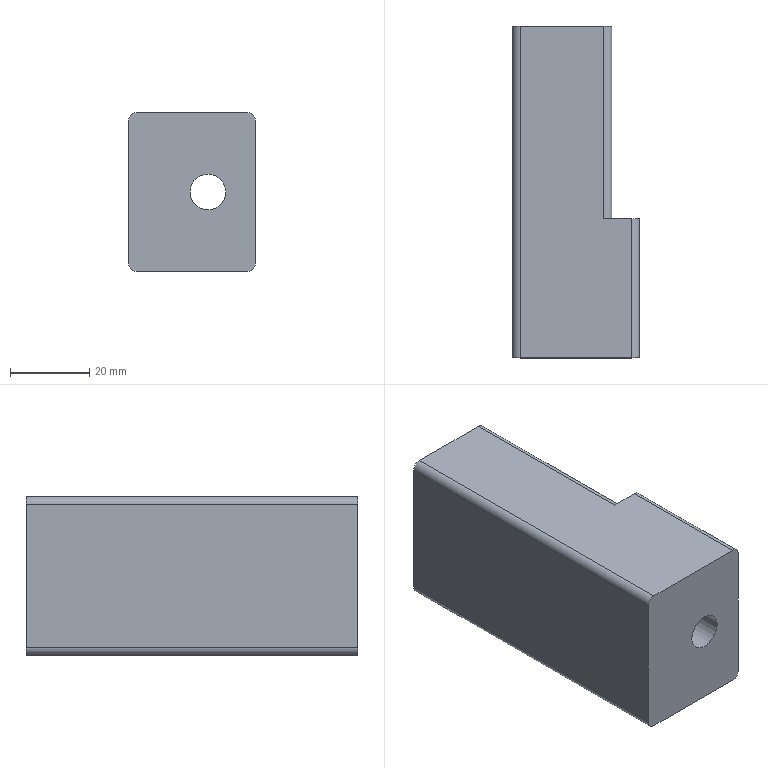CAM job | Mastercam | 3-axis milling, 5-axis milling, drilling | part box 32 x 83.5 x 40 mm | stock box 32 x 90 x 50 mm
Tools:
tool_number,name,type,diameter_mm,corner_radius_mm,flutes,flute_length_mm,overall_length_mm,shoulder_length_mm,holder_diameter_mm,length_offset,diameter_offset,default_rpm,default_feed_mm_min,default_plunge_mm_min,coolant
1,2 Flat End Mill,end mill,2,0,4,10,75,25,50,1,1,3500,500,600,COOL_OFF
5,4 Chamfer Mill,chamfer mill,4,0,4,25,75,30,50,5,5,7000,1000,600,COOL_OFF
7,6 Chamfer Mill,chamfer mill,6,0,4,25,100,30,50,7,7,5000,500,600,COOL_OFF
9,10 Flat End Mill,end mill,10,0,4,25,75,25,50,9,9,10000,5000,600,COOL_OFF
10,10 Flat End Mill,end mill,10,0,4,25,75,25,50,10,10,7000,1000,600,COOL_OFF
12,12 Flat End Mill,end mill,12,0,4,25,75,25,50,12,12,5000,500,600,COOL_OFF
15,3 Ball Mill / Bull Nose Mill,ball end mill,3,1.5,4,25,100,30,50,15,15,7000,1000,600,COOL_OFF
18,10 Bull Nose Mill,bull end mill,10,1,4,25,100,25,50,18,18,7000,3000,600,COOL_OFF
20,63 Flat End Mill,end mill,63,0,4,25,75,25,50,20,20,4000,1000,600,COOL_OFF
Operations:
seq,operation,operation_type,tool_number,tool_name,tool_diameter_mm,spindle_rpm,feed_mm_min,plunge_mm_min,retract_mm_min,cycle_time_s,wcs,posted,nc_file
1,Facing - [WCS: Plane-1] - [Tplane: Plane-1],Facing,20,63 Flat End Mill,63,4000,1000,600,1200,14.386,Plane-1,yes,.nc
2,Contour (Ramp) - [WCS: Plane-1] - [Tplane: Plane-1],Contour,9,10 Flat End Mill,10,10000,5000,600,1200,112.969,Plane-1,yes,.nc
3,Contour (2D) - [WCS: Plane-1] - [Tplane: Plane-1],Contour,10,10 Flat End Mill,10,7000,1000,600,1200,44.049,Plane-1,yes,.nc
4,Surface Finish Flowline - [WCS: Plane-1] - [Tplane: Plane-1],MultiSurfaceFinishFlowline,18,10 Bull Nose Mill,10,7000,3000,600,1200,133.321,Plane-1,yes,.nc
5,Deburr 5-axis - [WCS: Plane-1] - [Tplane: Plane-1],459,15,3 Ball Mill / Bull Nose Mill,3,7000,1000,600,1200,9.422,Plane-1,yes,.nc
6,Facing - [WCS: Plane-2] - [Tplane: Plane-2],Facing,20,63 Flat End Mill,63,4000,3000,600,1200,75.979,Plane-2,yes,.nc
7,Surface Finish Flowline - [WCS: Plane-2] - [Tplane: Plane-2],MultiSurfaceFinishFlowline,18,10 Bull Nose Mill,10,7000,3000,600,1200,65.421,Plane-2,yes,.nc
8,Deburr 5-axis - [WCS: Plane-2] - [Tplane: Plane-2],459,15,3 Ball Mill / Bull Nose Mill,3,7000,1000,600,1200,4.5,Plane-2,yes,.nc
9,Contour (2D chamfer) - [WCS: Plane-2] - [Tplane: Plane-2],Contour,5,4 Chamfer Mill,4,7000,1000,600,1200,13.32,Plane-2,yes,.nc
10,Drill/Counterbore - [WCS: Plane-4] - [Tplane: Plane-4],Drill,5,4 Chamfer Mill,4,3000,300,600,1200,0.819,Plane-4,yes,.nc
11,Contour (Ramp) - [WCS: Plane-5] - [Tplane: Plane-3],Contour,9,10 Flat End Mill,10,7000,3000,600,1200,110.155,Plane-5,yes,.nc
12,Contour (Ramp) - [WCS: Plane-5] - [Tplane: Plane-3],Contour,9,10 Flat End Mill,10,7000,3000,600,1200,168.554,Plane-5,yes,.nc
13,Contour (2D) - [WCS: Plane-5] - [Tplane: Plane-3],Contour,10,10 Flat End Mill,10,7000,1000,600,1200,21.928,Plane-5,yes,.nc
14,Contour (2D) - [WCS: Plane-5] - [Tplane: Plane-3],Contour,10,10 Flat End Mill,10,7000,1000,600,1200,33.618,Plane-5,yes,.nc
15,Contour (2D chamfer) - [WCS: Plane-5] - [Tplane: Plane-3],Contour,5,4 Chamfer Mill,4,7000,1000,600,1200,9.848,Plane-5,yes,.nc
16,Contour (Ramp) - [WCS: Plane-5] - [Tplane: Plane-3],Contour,12,12 Flat End Mill,12,5000,1000,600,1200,19.7,Plane-5,yes,.nc
17,Contour (2D) - [WCS: Plane-5] - [Tplane: Plane-3],Contour,12,12 Flat End Mill,12,5000,300,600,1200,8.928,Plane-5,yes,.nc
18,Contour (Ramp) - [WCS: Plane-5] - [Tplane: Plane-3],Contour,1,2 Flat End Mill,2,3500,500,600,1200,217.491,Plane-5,yes,.nc
19,Model Chamfer - [WCS: Plane-5] - [Tplane: Plane-3],ModelChamfer,7,6 Chamfer Mill,6,5000,500,600,1200,15.149,Plane-5,yes,.nc
20,Drill/Counterbore - [WCS: Plane-5] - [Tplane: Plane-3],Drill,7,6 Chamfer Mill,6,3000,300,600,1200,1.299,Plane-5,yes,.nc